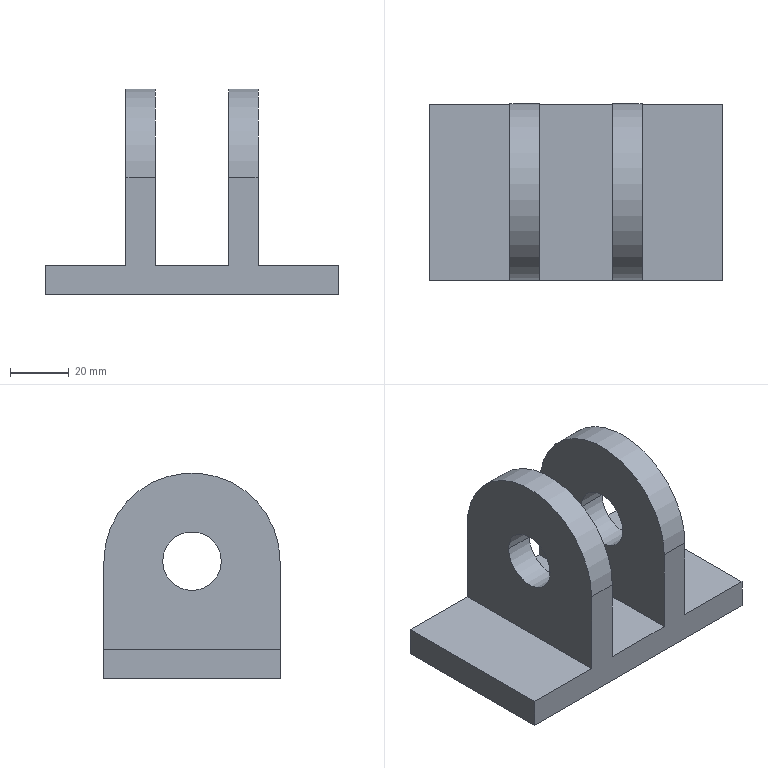Part | STEP file | FZC-000-003 Upper cylinder support | 1 solid | 18 faces | box 100 x 60 x 70 mm | volume 117991 mm3 | plane 12 | cylinder 6 | commonest cylinder face diameters 20 x4 60 x2
STEP:
#1=CARTESIAN_POINT('',(-4.67,0.3297,40.));
#2=VERTEX_POINT('',#1);
#3=CARTESIAN_POINT('',(-4.67,-19.67,40.));
#4=VERTEX_POINT('',#3);
#5=CARTESIAN_POINT('',(-4.67,-9.67,40.));
#6=DIRECTION('',(-1.,0.,0.));
#7=DIRECTION('',(0.,1.,0.));
#8=AXIS2_PLACEMENT_3D('',#5,#6,#7);
#9=CIRCLE('',#8,10.);
#10=EDGE_CURVE('',#2,#4,#9,.T.);
#11=ORIENTED_EDGE('',*,*,#10,.T.);
#12=CARTESIAN_POINT('',(5.33,-19.67,40.));
#13=VERTEX_POINT('',#12);
#14=CARTESIAN_POINT('',(-54.67,-19.67,40.));
#15=DIRECTION('',(1.,0.,0.));
#16=VECTOR('',#15,1000.);
#17=LINE('',#14,#16);
#18=EDGE_CURVE('',#4,#13,#17,.T.);
#19=ORIENTED_EDGE('',*,*,#18,.T.);
#20=CARTESIAN_POINT('',(5.33,0.3297,40.));
#21=VERTEX_POINT('',#20);
#22=CARTESIAN_POINT('',(5.33,-9.67,40.));
#23=DIRECTION('',(1.,0.,0.));
#24=DIRECTION('',(0.,1.,0.));
#25=AXIS2_PLACEMENT_3D('',#22,#23,#24);
#26=CIRCLE('',#25,10.);
#27=EDGE_CURVE('',#13,#21,#26,.T.);
#28=ORIENTED_EDGE('',*,*,#27,.T.);
#29=CARTESIAN_POINT('',(-54.67,0.3297,40.));
#30=DIRECTION('',(1.,0.,0.));
#31=VECTOR('',#30,1000.);
#32=LINE('',#29,#31);
#33=EDGE_CURVE('',#2,#21,#32,.T.);
#34=ORIENTED_EDGE('',*,*,#33,.F.);
#35=EDGE_LOOP('',(#11,#19,#28,#34));
#36=FACE_OUTER_BOUND('',#35,.T.);
#37=CARTESIAN_POINT('',(-54.67,-9.67,40.));
#38=DIRECTION('',(1.,0.,0.));
#39=DIRECTION('',(0.,1.,0.));
#40=AXIS2_PLACEMENT_3D('',#37,#38,#39);
#41=CYLINDRICAL_SURFACE('',#40,10.);
#42=ADVANCED_FACE('',(#36),#41,.F.);
#43=CARTESIAN_POINT('',(-39.67,0.3297,40.));
#44=VERTEX_POINT('',#43);
#45=CARTESIAN_POINT('',(-39.67,-19.67,40.));
#46=VERTEX_POINT('',#45);
#47=CARTESIAN_POINT('',(-39.67,-9.67,40.));
#48=DIRECTION('',(-1.,0.,0.));
#49=DIRECTION('',(0.,1.,0.));
#50=AXIS2_PLACEMENT_3D('',#47,#48,#49);
#51=CIRCLE('',#50,10.);
#52=EDGE_CURVE('',#44,#46,#51,.T.);
#53=ORIENTED_EDGE('',*,*,#52,.T.);
#54=CARTESIAN_POINT('',(-29.67,-19.67,40.));
#55=VERTEX_POINT('',#54);
#56=CARTESIAN_POINT('',(-54.67,-19.67,40.));
#57=DIRECTION('',(1.,0.,0.));
#58=VECTOR('',#57,1000.);
#59=LINE('',#56,#58);
#60=EDGE_CURVE('',#46,#55,#59,.T.);
#61=ORIENTED_EDGE('',*,*,#60,.T.);
#62=CARTESIAN_POINT('',(-29.67,0.3297,40.));
#63=VERTEX_POINT('',#62);
#64=CARTESIAN_POINT('',(-29.67,-9.67,40.));
#65=DIRECTION('',(1.,0.,0.));
#66=DIRECTION('',(0.,1.,0.));
#67=AXIS2_PLACEMENT_3D('',#64,#65,#66);
#68=CIRCLE('',#67,10.);
#69=EDGE_CURVE('',#55,#63,#68,.T.);
#70=ORIENTED_EDGE('',*,*,#69,.T.);
#71=CARTESIAN_POINT('',(-54.67,0.3297,40.));
#72=DIRECTION('',(1.,0.,0.));
#73=VECTOR('',#72,1000.);
#74=LINE('',#71,#73);
#75=EDGE_CURVE('',#44,#63,#74,.T.);
#76=ORIENTED_EDGE('',*,*,#75,.F.);
#77=EDGE_LOOP('',(#53,#61,#70,#76));
#78=FACE_OUTER_BOUND('',#77,.T.);
#79=CARTESIAN_POINT('',(-54.67,-9.67,40.));
#80=DIRECTION('',(1.,0.,0.));
#81=DIRECTION('',(0.,1.,0.));
#82=AXIS2_PLACEMENT_3D('',#79,#80,#81);
#83=CYLINDRICAL_SURFACE('',#82,10.);
#84=ADVANCED_FACE('',(#78),#83,.F.);
#85=CARTESIAN_POINT('',(32.83,20.33,0.));
#86=VERTEX_POINT('',#85);
#87=CARTESIAN_POINT('',(-67.17,20.33,0.));
#88=VERTEX_POINT('',#87);
#89=CARTESIAN_POINT('',(0.,20.33,0.));
#90=DIRECTION('',(-1.,0.,0.));
#91=VECTOR('',#90,1000.);
#92=LINE('',#89,#91);
#93=EDGE_CURVE('',#86,#88,#92,.T.);
#94=ORIENTED_EDGE('',*,*,#93,.F.);
#95=CARTESIAN_POINT('',(32.83,-39.67,0.));
#96=VERTEX_POINT('',#95);
#97=CARTESIAN_POINT('',(32.83,0.,0.));
#98=DIRECTION('',(0.,1.,0.));
#99=VECTOR('',#98,1000.);
#100=LINE('',#97,#99);
#101=EDGE_CURVE('',#96,#86,#100,.T.);
#102=ORIENTED_EDGE('',*,*,#101,.F.);
#103=CARTESIAN_POINT('',(-67.17,-39.67,0.));
#104=VERTEX_POINT('',#103);
#105=CARTESIAN_POINT('',(0.,-39.67,0.));
#106=DIRECTION('',(1.,0.,0.));
#107=VECTOR('',#106,1000.);
#108=LINE('',#105,#107);
#109=EDGE_CURVE('',#104,#96,#108,.T.);
#110=ORIENTED_EDGE('',*,*,#109,.F.);
#111=CARTESIAN_POINT('',(-67.17,0.,0.));
#112=DIRECTION('',(0.,-1.,0.));
#113=VECTOR('',#112,1000.);
#114=LINE('',#111,#113);
#115=EDGE_CURVE('',#88,#104,#114,.T.);
#116=ORIENTED_EDGE('',*,*,#115,.F.);
#117=EDGE_LOOP('',(#94,#102,#110,#116));
#118=FACE_OUTER_BOUND('',#117,.T.);
#119=CARTESIAN_POINT('',(0.,0.,0.));
#120=DIRECTION('',(0.,0.,1.));
#121=DIRECTION('',(1.,0.,0.));
#122=AXIS2_PLACEMENT_3D('',#119,#120,#121);
#123=PLANE('',#122);
#124=ADVANCED_FACE('',(#118),#123,.F.);
#125=CARTESIAN_POINT('',(-67.17,-39.67,10.));
#126=VERTEX_POINT('',#125);
#127=CARTESIAN_POINT('',(-67.17,-39.67,10.));
#128=DIRECTION('',(0.,0.,-1.));
#129=VECTOR('',#128,1000.);
#130=LINE('',#127,#129);
#131=EDGE_CURVE('',#126,#104,#130,.T.);
#132=ORIENTED_EDGE('',*,*,#131,.F.);
#133=CARTESIAN_POINT('',(-67.17,20.33,10.));
#134=VERTEX_POINT('',#133);
#135=CARTESIAN_POINT('',(-67.17,20.33,10.));
#136=DIRECTION('',(0.,-1.,0.));
#137=VECTOR('',#136,1000.);
#138=LINE('',#135,#137);
#139=EDGE_CURVE('',#134,#126,#138,.T.);
#140=ORIENTED_EDGE('',*,*,#139,.F.);
#141=CARTESIAN_POINT('',(-67.17,20.33,10.));
#142=DIRECTION('',(0.,0.,1.));
#143=VECTOR('',#142,1000.);
#144=LINE('',#141,#143);
#145=EDGE_CURVE('',#88,#134,#144,.T.);
#146=ORIENTED_EDGE('',*,*,#145,.F.);
#147=ORIENTED_EDGE('',*,*,#115,.T.);
#148=EDGE_LOOP('',(#132,#140,#146,#147));
#149=FACE_OUTER_BOUND('',#148,.T.);
#150=CARTESIAN_POINT('',(-67.17,20.33,10.));
#151=DIRECTION('',(1.,0.,0.));
#152=DIRECTION('',(0.,1.,0.));
#153=AXIS2_PLACEMENT_3D('',#150,#151,#152);
#154=PLANE('',#153);
#155=ADVANCED_FACE('',(#149),#154,.F.);
#156=CARTESIAN_POINT('',(5.33,20.33,40.));
#157=VERTEX_POINT('',#156);
#158=CARTESIAN_POINT('',(-4.67,20.33,40.));
#159=VERTEX_POINT('',#158);
#160=CARTESIAN_POINT('',(-67.17,20.33,40.));
#161=DIRECTION('',(-1.,0.,0.));
#162=VECTOR('',#161,1000.);
#163=LINE('',#160,#162);
#164=EDGE_CURVE('',#157,#159,#163,.T.);
#165=ORIENTED_EDGE('',*,*,#164,.F.);
#166=CARTESIAN_POINT('',(5.33,20.33,10.));
#167=VERTEX_POINT('',#166);
#168=CARTESIAN_POINT('',(5.33,20.33,10.));
#169=DIRECTION('',(0.,0.,1.));
#170=VECTOR('',#169,1000.);
#171=LINE('',#168,#170);
#172=EDGE_CURVE('',#167,#157,#171,.T.);
#173=ORIENTED_EDGE('',*,*,#172,.F.);
#174=CARTESIAN_POINT('',(32.83,20.33,10.));
#175=VERTEX_POINT('',#174);
#176=CARTESIAN_POINT('',(-67.17,20.33,10.));
#177=DIRECTION('',(-1.,0.,0.));
#178=VECTOR('',#177,1000.);
#179=LINE('',#176,#178);
#180=EDGE_CURVE('',#175,#167,#179,.T.);
#181=ORIENTED_EDGE('',*,*,#180,.F.);
#182=CARTESIAN_POINT('',(32.83,20.33,10.));
#183=DIRECTION('',(0.,0.,1.));
#184=VECTOR('',#183,1000.);
#185=LINE('',#182,#184);
#186=EDGE_CURVE('',#86,#175,#185,.T.);
#187=ORIENTED_EDGE('',*,*,#186,.F.);
#188=ORIENTED_EDGE('',*,*,#93,.T.);
#189=ORIENTED_EDGE('',*,*,#145,.T.);
#190=CARTESIAN_POINT('',(-39.67,20.33,10.));
#191=VERTEX_POINT('',#190);
#192=CARTESIAN_POINT('',(-67.17,20.33,10.));
#193=DIRECTION('',(-1.,0.,0.));
#194=VECTOR('',#193,1000.);
#195=LINE('',#192,#194);
#196=EDGE_CURVE('',#191,#134,#195,.T.);
#197=ORIENTED_EDGE('',*,*,#196,.F.);
#198=CARTESIAN_POINT('',(-39.67,20.33,40.));
#199=VERTEX_POINT('',#198);
#200=CARTESIAN_POINT('',(-39.67,20.33,10.));
#201=DIRECTION('',(0.,0.,-1.));
#202=VECTOR('',#201,1000.);
#203=LINE('',#200,#202);
#204=EDGE_CURVE('',#199,#191,#203,.T.);
#205=ORIENTED_EDGE('',*,*,#204,.F.);
#206=CARTESIAN_POINT('',(-29.67,20.33,40.));
#207=VERTEX_POINT('',#206);
#208=CARTESIAN_POINT('',(-67.17,20.33,40.));
#209=DIRECTION('',(-1.,0.,0.));
#210=VECTOR('',#209,1000.);
#211=LINE('',#208,#210);
#212=EDGE_CURVE('',#207,#199,#211,.T.);
#213=ORIENTED_EDGE('',*,*,#212,.F.);
#214=CARTESIAN_POINT('',(-29.67,20.33,10.));
#215=VERTEX_POINT('',#214);
#216=CARTESIAN_POINT('',(-29.67,20.33,10.));
#217=DIRECTION('',(0.,0.,1.));
#218=VECTOR('',#217,1000.);
#219=LINE('',#216,#218);
#220=EDGE_CURVE('',#215,#207,#219,.T.);
#221=ORIENTED_EDGE('',*,*,#220,.F.);
#222=CARTESIAN_POINT('',(-4.67,20.33,10.));
#223=VERTEX_POINT('',#222);
#224=CARTESIAN_POINT('',(-67.17,20.33,10.));
#225=DIRECTION('',(-1.,0.,0.));
#226=VECTOR('',#225,1000.);
#227=LINE('',#224,#226);
#228=EDGE_CURVE('',#223,#215,#227,.T.);
#229=ORIENTED_EDGE('',*,*,#228,.F.);
#230=CARTESIAN_POINT('',(-4.67,20.33,10.));
#231=DIRECTION('',(0.,0.,-1.));
#232=VECTOR('',#231,1000.);
#233=LINE('',#230,#232);
#234=EDGE_CURVE('',#159,#223,#233,.T.);
#235=ORIENTED_EDGE('',*,*,#234,.F.);
#236=EDGE_LOOP('',(#165,#173,#181,#187,#188,#189,#197,#205,#213,#221,#229,#235));
#237=FACE_OUTER_BOUND('',#236,.T.);
#238=CARTESIAN_POINT('',(-67.17,20.33,10.));
#239=DIRECTION('',(0.,-1.,0.));
#240=DIRECTION('',(0.,0.,-1.));
#241=AXIS2_PLACEMENT_3D('',#238,#239,#240);
#242=PLANE('',#241);
#243=ADVANCED_FACE('',(#237),#242,.F.);
#244=ORIENTED_EDGE('',*,*,#186,.T.);
#245=CARTESIAN_POINT('',(32.83,-39.67,10.));
#246=VERTEX_POINT('',#245);
#247=CARTESIAN_POINT('',(32.83,20.33,10.));
#248=DIRECTION('',(0.,1.,0.));
#249=VECTOR('',#248,1000.);
#250=LINE('',#247,#249);
#251=EDGE_CURVE('',#246,#175,#250,.T.);
#252=ORIENTED_EDGE('',*,*,#251,.F.);
#253=CARTESIAN_POINT('',(32.83,-39.67,10.));
#254=DIRECTION('',(0.,0.,1.));
#255=VECTOR('',#254,1000.);
#256=LINE('',#253,#255);
#257=EDGE_CURVE('',#96,#246,#256,.T.);
#258=ORIENTED_EDGE('',*,*,#257,.F.);
#259=ORIENTED_EDGE('',*,*,#101,.T.);
#260=EDGE_LOOP('',(#244,#252,#258,#259));
#261=FACE_OUTER_BOUND('',#260,.T.);
#262=CARTESIAN_POINT('',(32.83,20.33,10.));
#263=DIRECTION('',(-1.,0.,0.));
#264=DIRECTION('',(0.,-1.,0.));
#265=AXIS2_PLACEMENT_3D('',#262,#263,#264);
#266=PLANE('',#265);
#267=ADVANCED_FACE('',(#261),#266,.F.);
#268=CARTESIAN_POINT('',(-4.67,-39.67,40.));
#269=VERTEX_POINT('',#268);
#270=CARTESIAN_POINT('',(5.33,-39.67,40.));
#271=VERTEX_POINT('',#270);
#272=CARTESIAN_POINT('',(-67.17,-39.67,40.));
#273=DIRECTION('',(1.,0.,0.));
#274=VECTOR('',#273,1000.);
#275=LINE('',#272,#274);
#276=EDGE_CURVE('',#269,#271,#275,.T.);
#277=ORIENTED_EDGE('',*,*,#276,.F.);
#278=CARTESIAN_POINT('',(-4.67,-39.67,10.));
#279=VERTEX_POINT('',#278);
#280=CARTESIAN_POINT('',(-4.67,-39.67,10.));
#281=DIRECTION('',(0.,0.,1.));
#282=VECTOR('',#281,1000.);
#283=LINE('',#280,#282);
#284=EDGE_CURVE('',#279,#269,#283,.T.);
#285=ORIENTED_EDGE('',*,*,#284,.F.);
#286=CARTESIAN_POINT('',(-29.67,-39.67,10.));
#287=VERTEX_POINT('',#286);
#288=CARTESIAN_POINT('',(-67.17,-39.67,10.));
#289=DIRECTION('',(1.,0.,0.));
#290=VECTOR('',#289,1000.);
#291=LINE('',#288,#290);
#292=EDGE_CURVE('',#287,#279,#291,.T.);
#293=ORIENTED_EDGE('',*,*,#292,.F.);
#294=CARTESIAN_POINT('',(-29.67,-39.67,40.));
#295=VERTEX_POINT('',#294);
#296=CARTESIAN_POINT('',(-29.67,-39.67,10.));
#297=DIRECTION('',(0.,0.,-1.));
#298=VECTOR('',#297,1000.);
#299=LINE('',#296,#298);
#300=EDGE_CURVE('',#295,#287,#299,.T.);
#301=ORIENTED_EDGE('',*,*,#300,.F.);
#302=CARTESIAN_POINT('',(-39.67,-39.67,40.));
#303=VERTEX_POINT('',#302);
#304=CARTESIAN_POINT('',(-67.17,-39.67,40.));
#305=DIRECTION('',(1.,0.,0.));
#306=VECTOR('',#305,1000.);
#307=LINE('',#304,#306);
#308=EDGE_CURVE('',#303,#295,#307,.T.);
#309=ORIENTED_EDGE('',*,*,#308,.F.);
#310=CARTESIAN_POINT('',(-39.67,-39.67,10.));
#311=VERTEX_POINT('',#310);
#312=CARTESIAN_POINT('',(-39.67,-39.67,10.));
#313=DIRECTION('',(0.,0.,1.));
#314=VECTOR('',#313,1000.);
#315=LINE('',#312,#314);
#316=EDGE_CURVE('',#311,#303,#315,.T.);
#317=ORIENTED_EDGE('',*,*,#316,.F.);
#318=CARTESIAN_POINT('',(-67.17,-39.67,10.));
#319=DIRECTION('',(1.,0.,0.));
#320=VECTOR('',#319,1000.);
#321=LINE('',#318,#320);
#322=EDGE_CURVE('',#126,#311,#321,.T.);
#323=ORIENTED_EDGE('',*,*,#322,.F.);
#324=ORIENTED_EDGE('',*,*,#131,.T.);
#325=ORIENTED_EDGE('',*,*,#109,.T.);
#326=ORIENTED_EDGE('',*,*,#257,.T.);
#327=CARTESIAN_POINT('',(5.33,-39.67,10.));
#328=VERTEX_POINT('',#327);
#329=CARTESIAN_POINT('',(-67.17,-39.67,10.));
#330=DIRECTION('',(1.,0.,0.));
#331=VECTOR('',#330,1000.);
#332=LINE('',#329,#331);
#333=EDGE_CURVE('',#328,#246,#332,.T.);
#334=ORIENTED_EDGE('',*,*,#333,.F.);
#335=CARTESIAN_POINT('',(5.33,-39.67,10.));
#336=DIRECTION('',(0.,0.,-1.));
#337=VECTOR('',#336,1000.);
#338=LINE('',#335,#337);
#339=EDGE_CURVE('',#271,#328,#338,.T.);
#340=ORIENTED_EDGE('',*,*,#339,.F.);
#341=EDGE_LOOP('',(#277,#285,#293,#301,#309,#317,#323,#324,#325,#326,#334,#340));
#342=FACE_OUTER_BOUND('',#341,.T.);
#343=CARTESIAN_POINT('',(-67.17,-39.67,10.));
#344=DIRECTION('',(0.,1.,0.));
#345=DIRECTION('',(0.,0.,1.));
#346=AXIS2_PLACEMENT_3D('',#343,#344,#345);
#347=PLANE('',#346);
#348=ADVANCED_FACE('',(#342),#347,.F.);
#349=ORIENTED_EDGE('',*,*,#139,.T.);
#350=ORIENTED_EDGE('',*,*,#322,.T.);
#351=CARTESIAN_POINT('',(-39.67,0.,10.));
#352=DIRECTION('',(0.,1.,0.));
#353=VECTOR('',#352,1000.);
#354=LINE('',#351,#353);
#355=EDGE_CURVE('',#311,#191,#354,.T.);
#356=ORIENTED_EDGE('',*,*,#355,.T.);
#357=ORIENTED_EDGE('',*,*,#196,.T.);
#358=EDGE_LOOP('',(#349,#350,#356,#357));
#359=FACE_OUTER_BOUND('',#358,.T.);
#360=CARTESIAN_POINT('',(0.,0.,10.));
#361=DIRECTION('',(0.,0.,1.));
#362=DIRECTION('',(1.,0.,0.));
#363=AXIS2_PLACEMENT_3D('',#360,#361,#362);
#364=PLANE('',#363);
#365=ADVANCED_FACE('',(#359),#364,.T.);
#366=CARTESIAN_POINT('',(-4.67,-9.67,40.));
#367=DIRECTION('',(1.,0.,0.));
#368=DIRECTION('',(0.,0.,1.));
#369=AXIS2_PLACEMENT_3D('',#366,#367,#368);
#370=CIRCLE('',#369,30.);
#371=EDGE_CURVE('',#159,#269,#370,.T.);
#372=ORIENTED_EDGE('',*,*,#371,.F.);
#373=ORIENTED_EDGE('',*,*,#234,.T.);
#374=CARTESIAN_POINT('',(-4.67,20.33,10.));
#375=DIRECTION('',(0.,1.,0.));
#376=VECTOR('',#375,1000.);
#377=LINE('',#374,#376);
#378=EDGE_CURVE('',#279,#223,#377,.T.);
#379=ORIENTED_EDGE('',*,*,#378,.F.);
#380=ORIENTED_EDGE('',*,*,#284,.T.);
#381=EDGE_LOOP('',(#372,#373,#379,#380));
#382=FACE_OUTER_BOUND('',#381,.T.);
#383=ORIENTED_EDGE('',*,*,#10,.F.);
#384=CARTESIAN_POINT('',(-4.67,-9.67,40.));
#385=DIRECTION('',(-1.,0.,0.));
#386=DIRECTION('',(0.,1.,0.));
#387=AXIS2_PLACEMENT_3D('',#384,#385,#386);
#388=CIRCLE('',#387,10.);
#389=EDGE_CURVE('',#4,#2,#388,.T.);
#390=ORIENTED_EDGE('',*,*,#389,.F.);
#391=EDGE_LOOP('',(#383,#390));
#392=FACE_BOUND('',#391,.T.);
#393=CARTESIAN_POINT('',(-4.67,20.33,70.));
#394=DIRECTION('',(1.,0.,0.));
#395=DIRECTION('',(0.,1.,0.));
#396=AXIS2_PLACEMENT_3D('',#393,#394,#395);
#397=PLANE('',#396);
#398=ADVANCED_FACE('',(#382,#392),#397,.F.);
#399=ORIENTED_EDGE('',*,*,#164,.T.);
#400=ORIENTED_EDGE('',*,*,#371,.T.);
#401=ORIENTED_EDGE('',*,*,#276,.T.);
#402=CARTESIAN_POINT('',(5.33,-9.67,40.));
#403=DIRECTION('',(-1.,0.,0.));
#404=DIRECTION('',(0.,0.,-1.));
#405=AXIS2_PLACEMENT_3D('',#402,#403,#404);
#406=CIRCLE('',#405,30.);
#407=EDGE_CURVE('',#271,#157,#406,.T.);
#408=ORIENTED_EDGE('',*,*,#407,.T.);
#409=EDGE_LOOP('',(#399,#400,#401,#408));
#410=FACE_OUTER_BOUND('',#409,.T.);
#411=CARTESIAN_POINT('',(0.,-9.67,40.));
#412=DIRECTION('',(1.,0.,0.));
#413=DIRECTION('',(0.,0.,-1.));
#414=AXIS2_PLACEMENT_3D('',#411,#412,#413);
#415=CYLINDRICAL_SURFACE('',#414,30.);
#416=ADVANCED_FACE('',(#410),#415,.T.);
#417=ORIENTED_EDGE('',*,*,#407,.F.);
#418=ORIENTED_EDGE('',*,*,#339,.T.);
#419=CARTESIAN_POINT('',(5.33,20.33,10.));
#420=DIRECTION('',(0.,-1.,0.));
#421=VECTOR('',#420,1000.);
#422=LINE('',#419,#421);
#423=EDGE_CURVE('',#167,#328,#422,.T.);
#424=ORIENTED_EDGE('',*,*,#423,.F.);
#425=ORIENTED_EDGE('',*,*,#172,.T.);
#426=EDGE_LOOP('',(#417,#418,#424,#425));
#427=FACE_OUTER_BOUND('',#426,.T.);
#428=CARTESIAN_POINT('',(5.33,-9.67,40.));
#429=DIRECTION('',(1.,0.,0.));
#430=DIRECTION('',(0.,1.,0.));
#431=AXIS2_PLACEMENT_3D('',#428,#429,#430);
#432=CIRCLE('',#431,10.);
#433=EDGE_CURVE('',#21,#13,#432,.T.);
#434=ORIENTED_EDGE('',*,*,#433,.F.);
#435=ORIENTED_EDGE('',*,*,#27,.F.);
#436=EDGE_LOOP('',(#434,#435));
#437=FACE_BOUND('',#436,.T.);
#438=CARTESIAN_POINT('',(5.33,20.33,70.));
#439=DIRECTION('',(-1.,0.,0.));
#440=DIRECTION('',(0.,-1.,0.));
#441=AXIS2_PLACEMENT_3D('',#438,#439,#440);
#442=PLANE('',#441);
#443=ADVANCED_FACE('',(#427,#437),#442,.F.);
#444=ORIENTED_EDGE('',*,*,#333,.T.);
#445=ORIENTED_EDGE('',*,*,#251,.T.);
#446=ORIENTED_EDGE('',*,*,#180,.T.);
#447=ORIENTED_EDGE('',*,*,#423,.T.);
#448=EDGE_LOOP('',(#444,#445,#446,#447));
#449=FACE_OUTER_BOUND('',#448,.T.);
#450=CARTESIAN_POINT('',(0.,0.,10.));
#451=DIRECTION('',(0.,0.,1.));
#452=DIRECTION('',(1.,0.,0.));
#453=AXIS2_PLACEMENT_3D('',#450,#451,#452);
#454=PLANE('',#453);
#455=ADVANCED_FACE('',(#449),#454,.T.);
#456=CARTESIAN_POINT('',(-39.67,-9.67,40.));
#457=DIRECTION('',(1.,0.,0.));
#458=DIRECTION('',(0.,0.,1.));
#459=AXIS2_PLACEMENT_3D('',#456,#457,#458);
#460=CIRCLE('',#459,30.);
#461=EDGE_CURVE('',#199,#303,#460,.T.);
#462=ORIENTED_EDGE('',*,*,#461,.F.);
#463=ORIENTED_EDGE('',*,*,#204,.T.);
#464=ORIENTED_EDGE('',*,*,#355,.F.);
#465=ORIENTED_EDGE('',*,*,#316,.T.);
#466=EDGE_LOOP('',(#462,#463,#464,#465));
#467=FACE_OUTER_BOUND('',#466,.T.);
#468=ORIENTED_EDGE('',*,*,#52,.F.);
#469=CARTESIAN_POINT('',(-39.67,-9.67,40.));
#470=DIRECTION('',(-1.,0.,0.));
#471=DIRECTION('',(0.,1.,0.));
#472=AXIS2_PLACEMENT_3D('',#469,#470,#471);
#473=CIRCLE('',#472,10.);
#474=EDGE_CURVE('',#46,#44,#473,.T.);
#475=ORIENTED_EDGE('',*,*,#474,.F.);
#476=EDGE_LOOP('',(#468,#475));
#477=FACE_BOUND('',#476,.T.);
#478=CARTESIAN_POINT('',(-39.67,20.33,70.));
#479=DIRECTION('',(1.,0.,0.));
#480=DIRECTION('',(0.,1.,0.));
#481=AXIS2_PLACEMENT_3D('',#478,#479,#480);
#482=PLANE('',#481);
#483=ADVANCED_FACE('',(#467,#477),#482,.F.);
#484=ORIENTED_EDGE('',*,*,#212,.T.);
#485=ORIENTED_EDGE('',*,*,#461,.T.);
#486=ORIENTED_EDGE('',*,*,#308,.T.);
#487=CARTESIAN_POINT('',(-29.67,-9.67,40.));
#488=DIRECTION('',(-1.,0.,0.));
#489=DIRECTION('',(0.,0.,-1.));
#490=AXIS2_PLACEMENT_3D('',#487,#488,#489);
#491=CIRCLE('',#490,30.);
#492=EDGE_CURVE('',#295,#207,#491,.T.);
#493=ORIENTED_EDGE('',*,*,#492,.T.);
#494=EDGE_LOOP('',(#484,#485,#486,#493));
#495=FACE_OUTER_BOUND('',#494,.T.);
#496=CARTESIAN_POINT('',(0.,-9.67,40.));
#497=DIRECTION('',(1.,0.,0.));
#498=DIRECTION('',(0.,0.,-1.));
#499=AXIS2_PLACEMENT_3D('',#496,#497,#498);
#500=CYLINDRICAL_SURFACE('',#499,30.);
#501=ADVANCED_FACE('',(#495),#500,.T.);
#502=ORIENTED_EDGE('',*,*,#492,.F.);
#503=ORIENTED_EDGE('',*,*,#300,.T.);
#504=CARTESIAN_POINT('',(-29.67,20.33,10.));
#505=DIRECTION('',(0.,-1.,0.));
#506=VECTOR('',#505,1000.);
#507=LINE('',#504,#506);
#508=EDGE_CURVE('',#215,#287,#507,.T.);
#509=ORIENTED_EDGE('',*,*,#508,.F.);
#510=ORIENTED_EDGE('',*,*,#220,.T.);
#511=EDGE_LOOP('',(#502,#503,#509,#510));
#512=FACE_OUTER_BOUND('',#511,.T.);
#513=CARTESIAN_POINT('',(-29.67,-9.67,40.));
#514=DIRECTION('',(1.,0.,0.));
#515=DIRECTION('',(0.,1.,0.));
#516=AXIS2_PLACEMENT_3D('',#513,#514,#515);
#517=CIRCLE('',#516,10.);
#518=EDGE_CURVE('',#63,#55,#517,.T.);
#519=ORIENTED_EDGE('',*,*,#518,.F.);
#520=ORIENTED_EDGE('',*,*,#69,.F.);
#521=EDGE_LOOP('',(#519,#520));
#522=FACE_BOUND('',#521,.T.);
#523=CARTESIAN_POINT('',(-29.67,20.33,70.));
#524=DIRECTION('',(-1.,0.,0.));
#525=DIRECTION('',(0.,-1.,0.));
#526=AXIS2_PLACEMENT_3D('',#523,#524,#525);
#527=PLANE('',#526);
#528=ADVANCED_FACE('',(#512,#522),#527,.F.);
#529=ORIENTED_EDGE('',*,*,#228,.T.);
#530=ORIENTED_EDGE('',*,*,#508,.T.);
#531=ORIENTED_EDGE('',*,*,#292,.T.);
#532=ORIENTED_EDGE('',*,*,#378,.T.);
#533=EDGE_LOOP('',(#529,#530,#531,#532));
#534=FACE_OUTER_BOUND('',#533,.T.);
#535=CARTESIAN_POINT('',(0.,0.,10.));
#536=DIRECTION('',(0.,0.,1.));
#537=DIRECTION('',(1.,0.,0.));
#538=AXIS2_PLACEMENT_3D('',#535,#536,#537);
#539=PLANE('',#538);
#540=ADVANCED_FACE('',(#534),#539,.T.);
#541=ORIENTED_EDGE('',*,*,#18,.F.);
#542=ORIENTED_EDGE('',*,*,#389,.T.);
#543=ORIENTED_EDGE('',*,*,#33,.T.);
#544=ORIENTED_EDGE('',*,*,#433,.T.);
#545=EDGE_LOOP('',(#541,#542,#543,#544));
#546=FACE_OUTER_BOUND('',#545,.T.);
#547=CARTESIAN_POINT('',(-54.67,-9.67,40.));
#548=DIRECTION('',(1.,0.,0.));
#549=DIRECTION('',(0.,1.,0.));
#550=AXIS2_PLACEMENT_3D('',#547,#548,#549);
#551=CYLINDRICAL_SURFACE('',#550,10.);
#552=ADVANCED_FACE('',(#546),#551,.F.);
#553=ORIENTED_EDGE('',*,*,#60,.F.);
#554=ORIENTED_EDGE('',*,*,#474,.T.);
#555=ORIENTED_EDGE('',*,*,#75,.T.);
#556=ORIENTED_EDGE('',*,*,#518,.T.);
#557=EDGE_LOOP('',(#553,#554,#555,#556));
#558=FACE_OUTER_BOUND('',#557,.T.);
#559=CARTESIAN_POINT('',(-54.67,-9.67,40.));
#560=DIRECTION('',(1.,0.,0.));
#561=DIRECTION('',(0.,1.,0.));
#562=AXIS2_PLACEMENT_3D('',#559,#560,#561);
#563=CYLINDRICAL_SURFACE('',#562,10.);
#564=ADVANCED_FACE('',(#558),#563,.F.);
#565=CLOSED_SHELL('',(#42,#84,#124,#155,#243,#267,#348,#365,#398,#416,#443,#455,#483,#501,#528,#540,#552,#564));
#566=MANIFOLD_SOLID_BREP('',#565);
#567=CARTESIAN_POINT('',(0.,0.,0.));
#568=DIRECTION('',(0.,0.,1.));
#569=DIRECTION('',(1.,0.,0.));
#570=AXIS2_PLACEMENT_3D('',#567,#568,#569);
#571=(LENGTH_UNIT()NAMED_UNIT(*)SI_UNIT(.MILLI.,.METRE.));
#572=UNCERTAINTY_MEASURE_WITH_UNIT(LENGTH_MEASURE(0.00001),#571,'','');
#573=(NAMED_UNIT(*)PLANE_ANGLE_UNIT()SI_UNIT($,.RADIAN.));
#574=(NAMED_UNIT(*)SI_UNIT($,.STERADIAN.)SOLID_ANGLE_UNIT());
#575=(GEOMETRIC_REPRESENTATION_CONTEXT(3)GLOBAL_UNCERTAINTY_ASSIGNED_CONTEXT((#572))GLOBAL_UNIT_ASSIGNED_CONTEXT((#571,#573,#574))REPRESENTATION_CONTEXT('',''));
#576=ADVANCED_BREP_SHAPE_REPRESENTATION('',(#566,#570),#575);